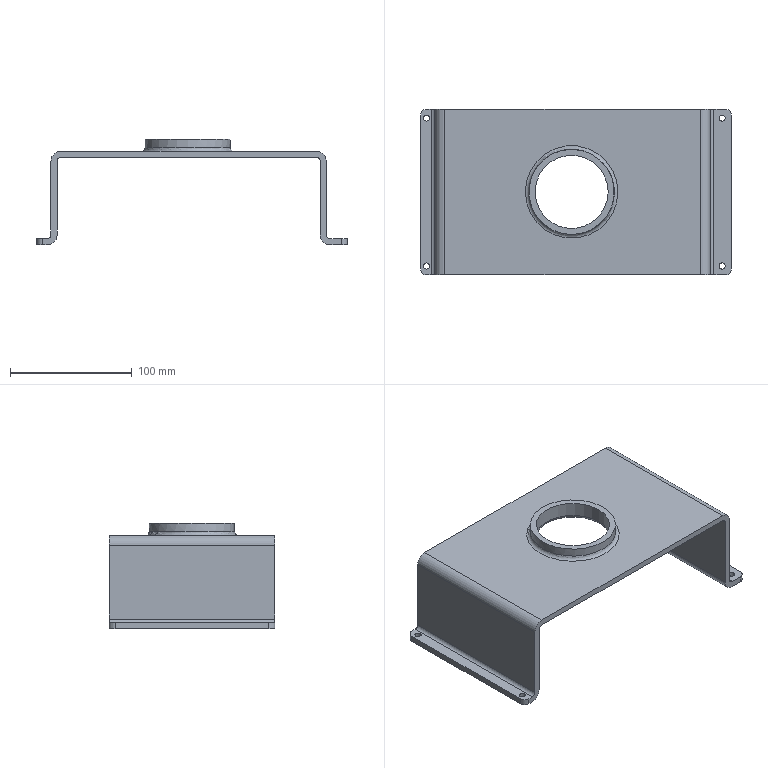Part | NX | features BREP 1 | 1 solid | 35 faces | box 255.4 x 136 x 86.7 mm | volume 260329 mm3 | cylinder 18 | plane 15 | torus 2 | commonest cylinder face diameters 5 x4 6 x4 10 x4 16 x4 60 x1 70 x1
STEP:
#1=CARTESIAN_POINT('',(38.,0.,5.));
#2=VERTEX_POINT('',#1);
#3=CARTESIAN_POINT('',(0.,0.,5.));
#4=DIRECTION('',(0.,0.,-1.));
#5=DIRECTION('',(1.,0.,0.));
#6=AXIS2_PLACEMENT_3D('',#3,#4,#5);
#7=CIRCLE('',#6,38.);
#8=EDGE_CURVE('',#2,#2,#7,.T.);
#9=ORIENTED_EDGE('',*,*,#8,.T.);
#10=EDGE_LOOP('',(#9));
#11=FACE_BOUND('',#10,.T.);
#12=CARTESIAN_POINT('',(-104.221,-68.,5.));
#13=VERTEX_POINT('',#12);
#14=CARTESIAN_POINT('',(105.779,-68.,5.));
#15=VERTEX_POINT('',#14);
#16=CARTESIAN_POINT('',(-124.221,-68.,5.));
#17=DIRECTION('',(1.,0.,0.));
#18=VECTOR('',#17,1000.);
#19=LINE('',#16,#18);
#20=EDGE_CURVE('',#13,#15,#19,.T.);
#21=ORIENTED_EDGE('',*,*,#20,.T.);
#22=CARTESIAN_POINT('',(105.779,68.,5.));
#23=VERTEX_POINT('',#22);
#24=CARTESIAN_POINT('',(105.779,-68.,5.));
#25=DIRECTION('',(0.,1.,0.));
#26=VECTOR('',#25,1000.);
#27=LINE('',#24,#26);
#28=EDGE_CURVE('',#15,#23,#27,.T.);
#29=ORIENTED_EDGE('',*,*,#28,.T.);
#30=CARTESIAN_POINT('',(-104.221,68.,5.));
#31=VERTEX_POINT('',#30);
#32=CARTESIAN_POINT('',(131.779,68.,5.));
#33=DIRECTION('',(-1.,0.,0.));
#34=VECTOR('',#33,1000.);
#35=LINE('',#32,#34);
#36=EDGE_CURVE('',#23,#31,#35,.T.);
#37=ORIENTED_EDGE('',*,*,#36,.T.);
#38=CARTESIAN_POINT('',(-104.221,68.,5.));
#39=DIRECTION('',(0.,-1.,0.));
#40=VECTOR('',#39,1000.);
#41=LINE('',#38,#40);
#42=EDGE_CURVE('',#31,#13,#41,.T.);
#43=ORIENTED_EDGE('',*,*,#42,.T.);
#44=EDGE_LOOP('',(#21,#29,#37,#43));
#45=FACE_BOUND('',#44,.T.);
#46=CARTESIAN_POINT('',(0.,0.,5.));
#47=DIRECTION('',(0.,0.,1.));
#48=DIRECTION('',(-1.,0.,0.));
#49=AXIS2_PLACEMENT_3D('',#46,#47,#48);
#50=PLANE('',#49);
#51=ADVANCED_FACE('',(#11,#45),#50,.T.);
#52=CARTESIAN_POINT('',(-115.221,68.,-71.7));
#53=VERTEX_POINT('',#52);
#54=CARTESIAN_POINT('',(-119.121,68.,-71.7));
#55=VERTEX_POINT('',#54);
#56=CARTESIAN_POINT('',(-115.221,68.,-71.7));
#57=DIRECTION('',(-1.,0.,0.));
#58=VECTOR('',#57,1000.);
#59=LINE('',#56,#58);
#60=EDGE_CURVE('',#53,#55,#59,.T.);
#61=ORIENTED_EDGE('',*,*,#60,.T.);
#62=CARTESIAN_POINT('',(-119.121,68.,-66.7));
#63=VERTEX_POINT('',#62);
#64=CARTESIAN_POINT('',(-119.121,68.,-66.7));
#65=DIRECTION('',(0.,0.,1.));
#66=VECTOR('',#65,1000.);
#67=LINE('',#64,#66);
#68=EDGE_CURVE('',#55,#63,#67,.T.);
#69=ORIENTED_EDGE('',*,*,#68,.T.);
#70=CARTESIAN_POINT('',(-115.221,68.,-66.7));
#71=VERTEX_POINT('',#70);
#72=CARTESIAN_POINT('',(-115.221,68.,-66.7));
#73=DIRECTION('',(-1.,0.,0.));
#74=VECTOR('',#73,1000.);
#75=LINE('',#72,#74);
#76=EDGE_CURVE('',#71,#63,#75,.T.);
#77=ORIENTED_EDGE('',*,*,#76,.F.);
#78=CARTESIAN_POINT('',(-112.221,68.,-63.7));
#79=VERTEX_POINT('',#78);
#80=CARTESIAN_POINT('',(-115.221,68.,-63.7));
#81=DIRECTION('',(0.,1.,0.));
#82=DIRECTION('',(1.,0.,0.));
#83=AXIS2_PLACEMENT_3D('',#80,#81,#82);
#84=CIRCLE('',#83,3.);
#85=EDGE_CURVE('',#79,#71,#84,.T.);
#86=ORIENTED_EDGE('',*,*,#85,.F.);
#87=CARTESIAN_POINT('',(-112.221,68.,-3.));
#88=VERTEX_POINT('',#87);
#89=CARTESIAN_POINT('',(-112.221,68.,-3.));
#90=DIRECTION('',(0.,0.,-1.));
#91=VECTOR('',#90,1000.);
#92=LINE('',#89,#91);
#93=EDGE_CURVE('',#88,#79,#92,.T.);
#94=ORIENTED_EDGE('',*,*,#93,.F.);
#95=CARTESIAN_POINT('',(-104.221,68.,-3.));
#96=DIRECTION('',(0.,-1.,0.));
#97=DIRECTION('',(-1.,0.,0.));
#98=AXIS2_PLACEMENT_3D('',#95,#96,#97);
#99=CIRCLE('',#98,8.);
#100=EDGE_CURVE('',#31,#88,#99,.T.);
#101=ORIENTED_EDGE('',*,*,#100,.F.);
#102=ORIENTED_EDGE('',*,*,#36,.F.);
#103=CARTESIAN_POINT('',(113.779,68.,-3.));
#104=VERTEX_POINT('',#103);
#105=CARTESIAN_POINT('',(105.779,68.,-3.));
#106=DIRECTION('',(0.,1.,0.));
#107=DIRECTION('',(1.,0.,0.));
#108=AXIS2_PLACEMENT_3D('',#105,#106,#107);
#109=CIRCLE('',#108,8.);
#110=EDGE_CURVE('',#23,#104,#109,.T.);
#111=ORIENTED_EDGE('',*,*,#110,.T.);
#112=CARTESIAN_POINT('',(113.779,68.,-63.6));
#113=VERTEX_POINT('',#112);
#114=CARTESIAN_POINT('',(113.779,68.,-3.));
#115=DIRECTION('',(0.,0.,-1.));
#116=VECTOR('',#115,1000.);
#117=LINE('',#114,#116);
#118=EDGE_CURVE('',#104,#113,#117,.T.);
#119=ORIENTED_EDGE('',*,*,#118,.T.);
#120=CARTESIAN_POINT('',(116.779,68.,-66.6));
#121=VERTEX_POINT('',#120);
#122=CARTESIAN_POINT('',(116.779,68.,-63.6));
#123=DIRECTION('',(0.,-1.,0.));
#124=DIRECTION('',(-1.,0.,0.));
#125=AXIS2_PLACEMENT_3D('',#122,#123,#124);
#126=CIRCLE('',#125,3.);
#127=EDGE_CURVE('',#113,#121,#126,.T.);
#128=ORIENTED_EDGE('',*,*,#127,.T.);
#129=CARTESIAN_POINT('',(126.279,68.,-66.6));
#130=VERTEX_POINT('',#129);
#131=CARTESIAN_POINT('',(116.779,68.,-66.6));
#132=DIRECTION('',(1.,0.,0.));
#133=VECTOR('',#132,1000.);
#134=LINE('',#131,#133);
#135=EDGE_CURVE('',#121,#130,#134,.T.);
#136=ORIENTED_EDGE('',*,*,#135,.T.);
#137=CARTESIAN_POINT('',(126.279,68.,-71.6));
#138=VERTEX_POINT('',#137);
#139=CARTESIAN_POINT('',(126.279,68.,-71.6));
#140=DIRECTION('',(0.,0.,-1.));
#141=VECTOR('',#140,1000.);
#142=LINE('',#139,#141);
#143=EDGE_CURVE('',#130,#138,#142,.T.);
#144=ORIENTED_EDGE('',*,*,#143,.T.);
#145=CARTESIAN_POINT('',(116.779,68.,-71.6));
#146=VERTEX_POINT('',#145);
#147=CARTESIAN_POINT('',(116.779,68.,-71.6));
#148=DIRECTION('',(1.,0.,0.));
#149=VECTOR('',#148,1000.);
#150=LINE('',#147,#149);
#151=EDGE_CURVE('',#146,#138,#150,.T.);
#152=ORIENTED_EDGE('',*,*,#151,.F.);
#153=CARTESIAN_POINT('',(108.779,68.,-63.6));
#154=VERTEX_POINT('',#153);
#155=CARTESIAN_POINT('',(116.779,68.,-63.6));
#156=DIRECTION('',(0.,-1.,0.));
#157=DIRECTION('',(-1.,0.,0.));
#158=AXIS2_PLACEMENT_3D('',#155,#156,#157);
#159=CIRCLE('',#158,8.);
#160=EDGE_CURVE('',#154,#146,#159,.T.);
#161=ORIENTED_EDGE('',*,*,#160,.F.);
#162=CARTESIAN_POINT('',(108.779,68.,-3.));
#163=VERTEX_POINT('',#162);
#164=CARTESIAN_POINT('',(108.779,68.,-3.));
#165=DIRECTION('',(0.,0.,-1.));
#166=VECTOR('',#165,1000.);
#167=LINE('',#164,#166);
#168=EDGE_CURVE('',#163,#154,#167,.T.);
#169=ORIENTED_EDGE('',*,*,#168,.F.);
#170=CARTESIAN_POINT('',(105.779,68.,0.));
#171=VERTEX_POINT('',#170);
#172=CARTESIAN_POINT('',(105.779,68.,-3.));
#173=DIRECTION('',(0.,1.,0.));
#174=DIRECTION('',(0.,0.,1.));
#175=AXIS2_PLACEMENT_3D('',#172,#173,#174);
#176=CIRCLE('',#175,3.);
#177=EDGE_CURVE('',#171,#163,#176,.T.);
#178=ORIENTED_EDGE('',*,*,#177,.F.);
#179=CARTESIAN_POINT('',(-104.221,68.,0.));
#180=VERTEX_POINT('',#179);
#181=CARTESIAN_POINT('',(0.,68.,0.));
#182=DIRECTION('',(-1.,0.,0.));
#183=VECTOR('',#182,1000.);
#184=LINE('',#181,#183);
#185=EDGE_CURVE('',#171,#180,#184,.T.);
#186=ORIENTED_EDGE('',*,*,#185,.T.);
#187=CARTESIAN_POINT('',(-107.221,68.,-3.));
#188=VERTEX_POINT('',#187);
#189=CARTESIAN_POINT('',(-104.221,68.,-3.));
#190=DIRECTION('',(0.,-1.,0.));
#191=DIRECTION('',(0.,0.,1.));
#192=AXIS2_PLACEMENT_3D('',#189,#190,#191);
#193=CIRCLE('',#192,3.);
#194=EDGE_CURVE('',#180,#188,#193,.T.);
#195=ORIENTED_EDGE('',*,*,#194,.T.);
#196=CARTESIAN_POINT('',(-107.221,68.,-63.7));
#197=VERTEX_POINT('',#196);
#198=CARTESIAN_POINT('',(-107.221,68.,-3.));
#199=DIRECTION('',(0.,0.,-1.));
#200=VECTOR('',#199,1000.);
#201=LINE('',#198,#200);
#202=EDGE_CURVE('',#188,#197,#201,.T.);
#203=ORIENTED_EDGE('',*,*,#202,.T.);
#204=CARTESIAN_POINT('',(-115.221,68.,-63.7));
#205=DIRECTION('',(0.,1.,0.));
#206=DIRECTION('',(1.,0.,0.));
#207=AXIS2_PLACEMENT_3D('',#204,#205,#206);
#208=CIRCLE('',#207,8.);
#209=EDGE_CURVE('',#197,#53,#208,.T.);
#210=ORIENTED_EDGE('',*,*,#209,.T.);
#211=EDGE_LOOP('',(#61,#69,#77,#86,#94,#101,#102,#111,#119,#128,#136,#144,#152,#161,#169,#178,#186,#195,#203,#210));
#212=FACE_BOUND('',#211,.T.);
#213=CARTESIAN_POINT('',(0.,68.,5.));
#214=DIRECTION('',(0.,-1.,0.));
#215=DIRECTION('',(-1.,0.,0.));
#216=AXIS2_PLACEMENT_3D('',#213,#214,#215);
#217=PLANE('',#216);
#218=ADVANCED_FACE('',(#212),#217,.F.);
#219=CARTESIAN_POINT('',(-115.221,-68.,-66.7));
#220=VERTEX_POINT('',#219);
#221=CARTESIAN_POINT('',(-119.121,-68.,-66.7));
#222=VERTEX_POINT('',#221);
#223=CARTESIAN_POINT('',(-115.221,-68.,-66.7));
#224=DIRECTION('',(-1.,0.,0.));
#225=VECTOR('',#224,1000.);
#226=LINE('',#223,#225);
#227=EDGE_CURVE('',#220,#222,#226,.T.);
#228=ORIENTED_EDGE('',*,*,#227,.T.);
#229=CARTESIAN_POINT('',(-119.121,-68.,-71.7));
#230=VERTEX_POINT('',#229);
#231=CARTESIAN_POINT('',(-119.121,-68.,-71.7));
#232=DIRECTION('',(0.,0.,-1.));
#233=VECTOR('',#232,1000.);
#234=LINE('',#231,#233);
#235=EDGE_CURVE('',#222,#230,#234,.T.);
#236=ORIENTED_EDGE('',*,*,#235,.T.);
#237=CARTESIAN_POINT('',(-115.221,-68.,-71.7));
#238=VERTEX_POINT('',#237);
#239=CARTESIAN_POINT('',(-115.221,-68.,-71.7));
#240=DIRECTION('',(-1.,0.,0.));
#241=VECTOR('',#240,1000.);
#242=LINE('',#239,#241);
#243=EDGE_CURVE('',#238,#230,#242,.T.);
#244=ORIENTED_EDGE('',*,*,#243,.F.);
#245=CARTESIAN_POINT('',(-107.221,-68.,-63.7));
#246=VERTEX_POINT('',#245);
#247=CARTESIAN_POINT('',(-115.221,-68.,-63.7));
#248=DIRECTION('',(0.,1.,0.));
#249=DIRECTION('',(1.,0.,0.));
#250=AXIS2_PLACEMENT_3D('',#247,#248,#249);
#251=CIRCLE('',#250,8.);
#252=EDGE_CURVE('',#246,#238,#251,.T.);
#253=ORIENTED_EDGE('',*,*,#252,.F.);
#254=CARTESIAN_POINT('',(-107.221,-68.,-3.));
#255=VERTEX_POINT('',#254);
#256=CARTESIAN_POINT('',(-107.221,-68.,-3.));
#257=DIRECTION('',(0.,0.,-1.));
#258=VECTOR('',#257,1000.);
#259=LINE('',#256,#258);
#260=EDGE_CURVE('',#255,#246,#259,.T.);
#261=ORIENTED_EDGE('',*,*,#260,.F.);
#262=CARTESIAN_POINT('',(-104.221,-68.,0.));
#263=VERTEX_POINT('',#262);
#264=CARTESIAN_POINT('',(-104.221,-68.,-3.));
#265=DIRECTION('',(0.,-1.,0.));
#266=DIRECTION('',(0.,0.,1.));
#267=AXIS2_PLACEMENT_3D('',#264,#265,#266);
#268=CIRCLE('',#267,3.);
#269=EDGE_CURVE('',#263,#255,#268,.T.);
#270=ORIENTED_EDGE('',*,*,#269,.F.);
#271=CARTESIAN_POINT('',(105.779,-68.,0.));
#272=VERTEX_POINT('',#271);
#273=CARTESIAN_POINT('',(-124.221,-68.,0.));
#274=DIRECTION('',(1.,0.,0.));
#275=VECTOR('',#274,1000.);
#276=LINE('',#273,#275);
#277=EDGE_CURVE('',#263,#272,#276,.T.);
#278=ORIENTED_EDGE('',*,*,#277,.T.);
#279=CARTESIAN_POINT('',(108.779,-68.,-3.));
#280=VERTEX_POINT('',#279);
#281=CARTESIAN_POINT('',(105.779,-68.,-3.));
#282=DIRECTION('',(0.,1.,0.));
#283=DIRECTION('',(0.,0.,1.));
#284=AXIS2_PLACEMENT_3D('',#281,#282,#283);
#285=CIRCLE('',#284,3.);
#286=EDGE_CURVE('',#272,#280,#285,.T.);
#287=ORIENTED_EDGE('',*,*,#286,.T.);
#288=CARTESIAN_POINT('',(108.779,-68.,-63.6));
#289=VERTEX_POINT('',#288);
#290=CARTESIAN_POINT('',(108.779,-68.,-3.));
#291=DIRECTION('',(0.,0.,-1.));
#292=VECTOR('',#291,1000.);
#293=LINE('',#290,#292);
#294=EDGE_CURVE('',#280,#289,#293,.T.);
#295=ORIENTED_EDGE('',*,*,#294,.T.);
#296=CARTESIAN_POINT('',(116.779,-68.,-71.6));
#297=VERTEX_POINT('',#296);
#298=CARTESIAN_POINT('',(116.779,-68.,-63.6));
#299=DIRECTION('',(0.,-1.,0.));
#300=DIRECTION('',(-1.,0.,0.));
#301=AXIS2_PLACEMENT_3D('',#298,#299,#300);
#302=CIRCLE('',#301,8.);
#303=EDGE_CURVE('',#289,#297,#302,.T.);
#304=ORIENTED_EDGE('',*,*,#303,.T.);
#305=CARTESIAN_POINT('',(126.279,-68.,-71.6));
#306=VERTEX_POINT('',#305);
#307=CARTESIAN_POINT('',(116.779,-68.,-71.6));
#308=DIRECTION('',(1.,0.,0.));
#309=VECTOR('',#308,1000.);
#310=LINE('',#307,#309);
#311=EDGE_CURVE('',#297,#306,#310,.T.);
#312=ORIENTED_EDGE('',*,*,#311,.T.);
#313=CARTESIAN_POINT('',(126.279,-68.,-66.6));
#314=VERTEX_POINT('',#313);
#315=CARTESIAN_POINT('',(126.279,-68.,-66.6));
#316=DIRECTION('',(0.,0.,1.));
#317=VECTOR('',#316,1000.);
#318=LINE('',#315,#317);
#319=EDGE_CURVE('',#306,#314,#318,.T.);
#320=ORIENTED_EDGE('',*,*,#319,.T.);
#321=CARTESIAN_POINT('',(116.779,-68.,-66.6));
#322=VERTEX_POINT('',#321);
#323=CARTESIAN_POINT('',(116.779,-68.,-66.6));
#324=DIRECTION('',(1.,0.,0.));
#325=VECTOR('',#324,1000.);
#326=LINE('',#323,#325);
#327=EDGE_CURVE('',#322,#314,#326,.T.);
#328=ORIENTED_EDGE('',*,*,#327,.F.);
#329=CARTESIAN_POINT('',(113.779,-68.,-63.6));
#330=VERTEX_POINT('',#329);
#331=CARTESIAN_POINT('',(116.779,-68.,-63.6));
#332=DIRECTION('',(0.,-1.,0.));
#333=DIRECTION('',(-1.,0.,0.));
#334=AXIS2_PLACEMENT_3D('',#331,#332,#333);
#335=CIRCLE('',#334,3.);
#336=EDGE_CURVE('',#330,#322,#335,.T.);
#337=ORIENTED_EDGE('',*,*,#336,.F.);
#338=CARTESIAN_POINT('',(113.779,-68.,-3.));
#339=VERTEX_POINT('',#338);
#340=CARTESIAN_POINT('',(113.779,-68.,-3.));
#341=DIRECTION('',(0.,0.,-1.));
#342=VECTOR('',#341,1000.);
#343=LINE('',#340,#342);
#344=EDGE_CURVE('',#339,#330,#343,.T.);
#345=ORIENTED_EDGE('',*,*,#344,.F.);
#346=CARTESIAN_POINT('',(105.779,-68.,-3.));
#347=DIRECTION('',(0.,1.,0.));
#348=DIRECTION('',(1.,0.,0.));
#349=AXIS2_PLACEMENT_3D('',#346,#347,#348);
#350=CIRCLE('',#349,8.);
#351=EDGE_CURVE('',#15,#339,#350,.T.);
#352=ORIENTED_EDGE('',*,*,#351,.F.);
#353=ORIENTED_EDGE('',*,*,#20,.F.);
#354=CARTESIAN_POINT('',(-112.221,-68.,-3.));
#355=VERTEX_POINT('',#354);
#356=CARTESIAN_POINT('',(-104.221,-68.,-3.));
#357=DIRECTION('',(0.,-1.,0.));
#358=DIRECTION('',(-1.,0.,0.));
#359=AXIS2_PLACEMENT_3D('',#356,#357,#358);
#360=CIRCLE('',#359,8.);
#361=EDGE_CURVE('',#13,#355,#360,.T.);
#362=ORIENTED_EDGE('',*,*,#361,.T.);
#363=CARTESIAN_POINT('',(-112.221,-68.,-63.7));
#364=VERTEX_POINT('',#363);
#365=CARTESIAN_POINT('',(-112.221,-68.,-3.));
#366=DIRECTION('',(0.,0.,-1.));
#367=VECTOR('',#366,1000.);
#368=LINE('',#365,#367);
#369=EDGE_CURVE('',#355,#364,#368,.T.);
#370=ORIENTED_EDGE('',*,*,#369,.T.);
#371=CARTESIAN_POINT('',(-115.221,-68.,-63.7));
#372=DIRECTION('',(0.,1.,0.));
#373=DIRECTION('',(1.,0.,0.));
#374=AXIS2_PLACEMENT_3D('',#371,#372,#373);
#375=CIRCLE('',#374,3.);
#376=EDGE_CURVE('',#364,#220,#375,.T.);
#377=ORIENTED_EDGE('',*,*,#376,.T.);
#378=EDGE_LOOP('',(#228,#236,#244,#253,#261,#270,#278,#287,#295,#304,#312,#320,#328,#337,#345,#352,#353,#362,#370,#377));
#379=FACE_BOUND('',#378,.T.);
#380=CARTESIAN_POINT('',(-124.221,-68.,5.));
#381=DIRECTION('',(0.,1.,0.));
#382=DIRECTION('',(1.,0.,0.));
#383=AXIS2_PLACEMENT_3D('',#380,#381,#382);
#384=PLANE('',#383);
#385=ADVANCED_FACE('',(#379),#384,.F.);
#386=CARTESIAN_POINT('',(33.,0.,0.));
#387=VERTEX_POINT('',#386);
#388=CARTESIAN_POINT('',(0.,0.,0.));
#389=DIRECTION('',(0.,0.,1.));
#390=DIRECTION('',(1.,0.,0.));
#391=AXIS2_PLACEMENT_3D('',#388,#389,#390);
#392=CIRCLE('',#391,33.);
#393=EDGE_CURVE('',#387,#387,#392,.T.);
#394=ORIENTED_EDGE('',*,*,#393,.T.);
#395=EDGE_LOOP('',(#394));
#396=FACE_BOUND('',#395,.T.);
#397=CARTESIAN_POINT('',(105.779,-68.,0.));
#398=DIRECTION('',(0.,1.,0.));
#399=VECTOR('',#398,1000.);
#400=LINE('',#397,#399);
#401=EDGE_CURVE('',#272,#171,#400,.T.);
#402=ORIENTED_EDGE('',*,*,#401,.F.);
#403=ORIENTED_EDGE('',*,*,#277,.F.);
#404=CARTESIAN_POINT('',(-104.221,68.,0.));
#405=DIRECTION('',(0.,-1.,0.));
#406=VECTOR('',#405,1000.);
#407=LINE('',#404,#406);
#408=EDGE_CURVE('',#180,#263,#407,.T.);
#409=ORIENTED_EDGE('',*,*,#408,.F.);
#410=ORIENTED_EDGE('',*,*,#185,.F.);
#411=EDGE_LOOP('',(#402,#403,#409,#410));
#412=FACE_BOUND('',#411,.T.);
#413=CARTESIAN_POINT('',(0.,0.,0.));
#414=DIRECTION('',(0.,0.,1.));
#415=DIRECTION('',(-1.,0.,0.));
#416=AXIS2_PLACEMENT_3D('',#413,#414,#415);
#417=PLANE('',#416);
#418=ADVANCED_FACE('',(#396,#412),#417,.F.);
#419=ORIENTED_EDGE('',*,*,#286,.F.);
#420=ORIENTED_EDGE('',*,*,#401,.T.);
#421=ORIENTED_EDGE('',*,*,#177,.T.);
#422=CARTESIAN_POINT('',(108.779,68.,-3.));
#423=DIRECTION('',(0.,-1.,0.));
#424=VECTOR('',#423,1000.);
#425=LINE('',#422,#424);
#426=EDGE_CURVE('',#163,#280,#425,.T.);
#427=ORIENTED_EDGE('',*,*,#426,.T.);
#428=EDGE_LOOP('',(#419,#420,#421,#427));
#429=FACE_BOUND('',#428,.T.);
#430=CARTESIAN_POINT('',(105.779,68.,-3.));
#431=DIRECTION('',(0.,-1.,0.));
#432=DIRECTION('',(-1.,0.,0.));
#433=AXIS2_PLACEMENT_3D('',#430,#431,#432);
#434=CYLINDRICAL_SURFACE('',#433,3.);
#435=ADVANCED_FACE('',(#429),#434,.F.);
#436=ORIENTED_EDGE('',*,*,#294,.F.);
#437=ORIENTED_EDGE('',*,*,#426,.F.);
#438=ORIENTED_EDGE('',*,*,#168,.T.);
#439=CARTESIAN_POINT('',(108.779,68.,-63.6));
#440=DIRECTION('',(0.,-1.,0.));
#441=VECTOR('',#440,1000.);
#442=LINE('',#439,#441);
#443=EDGE_CURVE('',#154,#289,#442,.T.);
#444=ORIENTED_EDGE('',*,*,#443,.T.);
#445=EDGE_LOOP('',(#436,#437,#438,#444));
#446=FACE_BOUND('',#445,.T.);
#447=CARTESIAN_POINT('',(108.779,68.,-3.));
#448=DIRECTION('',(-1.,0.,0.));
#449=DIRECTION('',(0.,1.,0.));
#450=AXIS2_PLACEMENT_3D('',#447,#448,#449);
#451=PLANE('',#450);
#452=ADVANCED_FACE('',(#446),#451,.T.);
#453=ORIENTED_EDGE('',*,*,#351,.T.);
#454=CARTESIAN_POINT('',(113.779,68.,-3.));
#455=DIRECTION('',(0.,-1.,0.));
#456=VECTOR('',#455,1000.);
#457=LINE('',#454,#456);
#458=EDGE_CURVE('',#104,#339,#457,.T.);
#459=ORIENTED_EDGE('',*,*,#458,.F.);
#460=ORIENTED_EDGE('',*,*,#110,.F.);
#461=ORIENTED_EDGE('',*,*,#28,.F.);
#462=EDGE_LOOP('',(#453,#459,#460,#461));
#463=FACE_BOUND('',#462,.T.);
#464=CARTESIAN_POINT('',(105.779,68.,-3.));
#465=DIRECTION('',(0.,-1.,0.));
#466=DIRECTION('',(-1.,0.,0.));
#467=AXIS2_PLACEMENT_3D('',#464,#465,#466);
#468=CYLINDRICAL_SURFACE('',#467,8.);
#469=ADVANCED_FACE('',(#463),#468,.T.);
#470=ORIENTED_EDGE('',*,*,#344,.T.);
#471=CARTESIAN_POINT('',(113.779,68.,-63.6));
#472=DIRECTION('',(0.,-1.,0.));
#473=VECTOR('',#472,1000.);
#474=LINE('',#471,#473);
#475=EDGE_CURVE('',#113,#330,#474,.T.);
#476=ORIENTED_EDGE('',*,*,#475,.F.);
#477=ORIENTED_EDGE('',*,*,#118,.F.);
#478=ORIENTED_EDGE('',*,*,#458,.T.);
#479=EDGE_LOOP('',(#470,#476,#477,#478));
#480=FACE_BOUND('',#479,.T.);
#481=CARTESIAN_POINT('',(113.779,68.,-3.));
#482=DIRECTION('',(-1.,0.,0.));
#483=DIRECTION('',(0.,1.,0.));
#484=AXIS2_PLACEMENT_3D('',#481,#482,#483);
#485=PLANE('',#484);
#486=ADVANCED_FACE('',(#480),#485,.F.);
#487=ORIENTED_EDGE('',*,*,#194,.F.);
#488=ORIENTED_EDGE('',*,*,#408,.T.);
#489=ORIENTED_EDGE('',*,*,#269,.T.);
#490=CARTESIAN_POINT('',(-107.221,-68.,-3.));
#491=DIRECTION('',(0.,1.,0.));
#492=VECTOR('',#491,1000.);
#493=LINE('',#490,#492);
#494=EDGE_CURVE('',#255,#188,#493,.T.);
#495=ORIENTED_EDGE('',*,*,#494,.T.);
#496=EDGE_LOOP('',(#487,#488,#489,#495));
#497=FACE_BOUND('',#496,.T.);
#498=CARTESIAN_POINT('',(-104.221,-68.,-3.));
#499=DIRECTION('',(0.,1.,0.));
#500=DIRECTION('',(1.,0.,0.));
#501=AXIS2_PLACEMENT_3D('',#498,#499,#500);
#502=CYLINDRICAL_SURFACE('',#501,3.);
#503=ADVANCED_FACE('',(#497),#502,.F.);
#504=ORIENTED_EDGE('',*,*,#202,.F.);
#505=ORIENTED_EDGE('',*,*,#494,.F.);
#506=ORIENTED_EDGE('',*,*,#260,.T.);
#507=CARTESIAN_POINT('',(-107.221,-68.,-63.7));
#508=DIRECTION('',(0.,1.,0.));
#509=VECTOR('',#508,1000.);
#510=LINE('',#507,#509);
#511=EDGE_CURVE('',#246,#197,#510,.T.);
#512=ORIENTED_EDGE('',*,*,#511,.T.);
#513=EDGE_LOOP('',(#504,#505,#506,#512));
#514=FACE_BOUND('',#513,.T.);
#515=CARTESIAN_POINT('',(-107.221,-68.,-3.));
#516=DIRECTION('',(1.,0.,0.));
#517=DIRECTION('',(0.,-1.,0.));
#518=AXIS2_PLACEMENT_3D('',#515,#516,#517);
#519=PLANE('',#518);
#520=ADVANCED_FACE('',(#514),#519,.T.);
#521=ORIENTED_EDGE('',*,*,#100,.T.);
#522=CARTESIAN_POINT('',(-112.221,-68.,-3.));
#523=DIRECTION('',(0.,1.,0.));
#524=VECTOR('',#523,1000.);
#525=LINE('',#522,#524);
#526=EDGE_CURVE('',#355,#88,#525,.T.);
#527=ORIENTED_EDGE('',*,*,#526,.F.);
#528=ORIENTED_EDGE('',*,*,#361,.F.);
#529=ORIENTED_EDGE('',*,*,#42,.F.);
#530=EDGE_LOOP('',(#521,#527,#528,#529));
#531=FACE_BOUND('',#530,.T.);
#532=CARTESIAN_POINT('',(-104.221,-68.,-3.));
#533=DIRECTION('',(0.,1.,0.));
#534=DIRECTION('',(1.,0.,0.));
#535=AXIS2_PLACEMENT_3D('',#532,#533,#534);
#536=CYLINDRICAL_SURFACE('',#535,8.);
#537=ADVANCED_FACE('',(#531),#536,.T.);
#538=ORIENTED_EDGE('',*,*,#93,.T.);
#539=CARTESIAN_POINT('',(-112.221,-68.,-63.7));
#540=DIRECTION('',(0.,1.,0.));
#541=VECTOR('',#540,1000.);
#542=LINE('',#539,#541);
#543=EDGE_CURVE('',#364,#79,#542,.T.);
#544=ORIENTED_EDGE('',*,*,#543,.F.);
#545=ORIENTED_EDGE('',*,*,#369,.F.);
#546=ORIENTED_EDGE('',*,*,#526,.T.);
#547=EDGE_LOOP('',(#538,#544,#545,#546));
#548=FACE_BOUND('',#547,.T.);
#549=CARTESIAN_POINT('',(-112.221,-68.,-3.));
#550=DIRECTION('',(1.,0.,0.));
#551=DIRECTION('',(0.,-1.,0.));
#552=AXIS2_PLACEMENT_3D('',#549,#550,#551);
#553=PLANE('',#552);
#554=ADVANCED_FACE('',(#548),#553,.F.);
#555=CARTESIAN_POINT('',(131.279,-63.,-66.6));
#556=VERTEX_POINT('',#555);
#557=CARTESIAN_POINT('',(131.279,63.,-66.6));
#558=VERTEX_POINT('',#557);
#559=CARTESIAN_POINT('',(131.279,-68.,-66.6));
#560=DIRECTION('',(0.,1.,0.));
#561=VECTOR('',#560,1000.);
#562=LINE('',#559,#561);
#563=EDGE_CURVE('',#556,#558,#562,.T.);
#564=ORIENTED_EDGE('',*,*,#563,.F.);
#565=CARTESIAN_POINT('',(131.279,-63.,-71.6));
#566=VERTEX_POINT('',#565);
#567=CARTESIAN_POINT('',(131.279,-63.,-71.6));
#568=DIRECTION('',(0.,0.,-1.));
#569=VECTOR('',#568,1000.);
#570=LINE('',#567,#569);
#571=EDGE_CURVE('',#556,#566,#570,.T.);
#572=ORIENTED_EDGE('',*,*,#571,.T.);
#573=CARTESIAN_POINT('',(131.279,63.,-71.6));
#574=VERTEX_POINT('',#573);
#575=CARTESIAN_POINT('',(131.279,-68.,-71.6));
#576=DIRECTION('',(0.,1.,0.));
#577=VECTOR('',#576,1000.);
#578=LINE('',#575,#577);
#579=EDGE_CURVE('',#566,#574,#578,.T.);
#580=ORIENTED_EDGE('',*,*,#579,.T.);
#581=CARTESIAN_POINT('',(131.279,63.,-66.6));
#582=DIRECTION('',(0.,0.,1.));
#583=VECTOR('',#582,1000.);
#584=LINE('',#581,#583);
#585=EDGE_CURVE('',#574,#558,#584,.T.);
#586=ORIENTED_EDGE('',*,*,#585,.T.);
#587=EDGE_LOOP('',(#564,#572,#580,#586));
#588=FACE_BOUND('',#587,.T.);
#589=CARTESIAN_POINT('',(131.279,-68.,-66.6));
#590=DIRECTION('',(1.,0.,0.));
#591=DIRECTION('',(0.,-1.,0.));
#592=AXIS2_PLACEMENT_3D('',#589,#590,#591);
#593=PLANE('',#592);
#594=ADVANCED_FACE('',(#588),#593,.T.);
#595=ORIENTED_EDGE('',*,*,#127,.F.);
#596=ORIENTED_EDGE('',*,*,#475,.T.);
#597=ORIENTED_EDGE('',*,*,#336,.T.);
#598=CARTESIAN_POINT('',(116.779,-68.,-66.6));
#599=DIRECTION('',(0.,1.,0.));
#600=VECTOR('',#599,1000.);
#601=LINE('',#598,#600);
#602=EDGE_CURVE('',#322,#121,#601,.T.);
#603=ORIENTED_EDGE('',*,*,#602,.T.);
#604=EDGE_LOOP('',(#595,#596,#597,#603));
#605=FACE_BOUND('',#604,.T.);
#606=CARTESIAN_POINT('',(116.779,-68.,-63.6));
#607=DIRECTION('',(0.,1.,0.));
#608=DIRECTION('',(1.,0.,0.));
#609=AXIS2_PLACEMENT_3D('',#606,#607,#608);
#610=CYLINDRICAL_SURFACE('',#609,3.);
#611=ADVANCED_FACE('',(#605),#610,.F.);
#612=CARTESIAN_POINT('',(126.047,-60.702,-66.6));
#613=VERTEX_POINT('',#612);
#614=CARTESIAN_POINT('',(123.547,-60.702,-66.6));
#615=DIRECTION('',(0.,0.,1.));
#616=DIRECTION('',(1.,0.,0.));
#617=AXIS2_PLACEMENT_3D('',#614,#615,#616);
#618=CIRCLE('',#617,2.5);
#619=EDGE_CURVE('',#613,#613,#618,.T.);
#620=ORIENTED_EDGE('',*,*,#619,.F.);
#621=EDGE_LOOP('',(#620));
#622=FACE_BOUND('',#621,.T.);
#623=CARTESIAN_POINT('',(126.047,60.702,-66.6));
#624=VERTEX_POINT('',#623);
#625=CARTESIAN_POINT('',(123.547,60.702,-66.6));
#626=DIRECTION('',(0.,0.,1.));
#627=DIRECTION('',(1.,0.,0.));
#628=AXIS2_PLACEMENT_3D('',#625,#626,#627);
#629=CIRCLE('',#628,2.5);
#630=EDGE_CURVE('',#624,#624,#629,.T.);
#631=ORIENTED_EDGE('',*,*,#630,.F.);
#632=EDGE_LOOP('',(#631));
#633=FACE_BOUND('',#632,.T.);
#634=ORIENTED_EDGE('',*,*,#327,.T.);
#635=CARTESIAN_POINT('',(126.279,-63.,-66.6));
#636=DIRECTION('',(0.,0.,1.));
#637=DIRECTION('',(1.,0.,0.));
#638=AXIS2_PLACEMENT_3D('',#635,#636,#637);
#639=CIRCLE('',#638,5.);
#640=EDGE_CURVE('',#314,#556,#639,.T.);
#641=ORIENTED_EDGE('',*,*,#640,.T.);
#642=ORIENTED_EDGE('',*,*,#563,.T.);
#643=CARTESIAN_POINT('',(126.279,63.,-66.6));
#644=DIRECTION('',(0.,0.,1.));
#645=DIRECTION('',(1.,0.,0.));
#646=AXIS2_PLACEMENT_3D('',#643,#644,#645);
#647=CIRCLE('',#646,5.);
#648=EDGE_CURVE('',#558,#130,#647,.T.);
#649=ORIENTED_EDGE('',*,*,#648,.T.);
#650=ORIENTED_EDGE('',*,*,#135,.F.);
#651=ORIENTED_EDGE('',*,*,#602,.F.);
#652=EDGE_LOOP('',(#634,#641,#642,#649,#650,#651));
#653=FACE_BOUND('',#652,.T.);
#654=CARTESIAN_POINT('',(116.779,-68.,-66.6));
#655=DIRECTION('',(0.,0.,1.));
#656=DIRECTION('',(-1.,0.,0.));
#657=AXIS2_PLACEMENT_3D('',#654,#655,#656);
#658=PLANE('',#657);
#659=ADVANCED_FACE('',(#622,#633,#653),#658,.T.);
#660=ORIENTED_EDGE('',*,*,#160,.T.);
#661=CARTESIAN_POINT('',(116.779,-68.,-71.6));
#662=DIRECTION('',(0.,1.,0.));
#663=VECTOR('',#662,1000.);
#664=LINE('',#661,#663);
#665=EDGE_CURVE('',#297,#146,#664,.T.);
#666=ORIENTED_EDGE('',*,*,#665,.F.);
#667=ORIENTED_EDGE('',*,*,#303,.F.);
#668=ORIENTED_EDGE('',*,*,#443,.F.);
#669=EDGE_LOOP('',(#660,#666,#667,#668));
#670=FACE_BOUND('',#669,.T.);
#671=CARTESIAN_POINT('',(116.779,-68.,-63.6));
#672=DIRECTION('',(0.,1.,0.));
#673=DIRECTION('',(1.,0.,0.));
#674=AXIS2_PLACEMENT_3D('',#671,#672,#673);
#675=CYLINDRICAL_SURFACE('',#674,8.);
#676=ADVANCED_FACE('',(#670),#675,.T.);
#677=CARTESIAN_POINT('',(126.047,-60.702,-71.6));
#678=VERTEX_POINT('',#677);
#679=CARTESIAN_POINT('',(123.547,-60.702,-71.6));
#680=DIRECTION('',(0.,0.,1.));
#681=DIRECTION('',(1.,0.,0.));
#682=AXIS2_PLACEMENT_3D('',#679,#680,#681);
#683=CIRCLE('',#682,2.5);
#684=EDGE_CURVE('',#678,#678,#683,.T.);
#685=ORIENTED_EDGE('',*,*,#684,.T.);
#686=EDGE_LOOP('',(#685));
#687=FACE_BOUND('',#686,.T.);
#688=CARTESIAN_POINT('',(126.047,60.702,-71.6));
#689=VERTEX_POINT('',#688);
#690=CARTESIAN_POINT('',(123.547,60.702,-71.6));
#691=DIRECTION('',(0.,0.,1.));
#692=DIRECTION('',(1.,0.,0.));
#693=AXIS2_PLACEMENT_3D('',#690,#691,#692);
#694=CIRCLE('',#693,2.5);
#695=EDGE_CURVE('',#689,#689,#694,.T.);
#696=ORIENTED_EDGE('',*,*,#695,.T.);
#697=EDGE_LOOP('',(#696));
#698=FACE_BOUND('',#697,.T.);
#699=ORIENTED_EDGE('',*,*,#579,.F.);
#700=CARTESIAN_POINT('',(126.279,-63.,-71.6));
#701=DIRECTION('',(0.,0.,-1.));
#702=DIRECTION('',(1.,0.,0.));
#703=AXIS2_PLACEMENT_3D('',#700,#701,#702);
#704=CIRCLE('',#703,5.);
#705=EDGE_CURVE('',#566,#306,#704,.T.);
#706=ORIENTED_EDGE('',*,*,#705,.T.);
#707=ORIENTED_EDGE('',*,*,#311,.F.);
#708=ORIENTED_EDGE('',*,*,#665,.T.);
#709=ORIENTED_EDGE('',*,*,#151,.T.);
#710=CARTESIAN_POINT('',(126.279,63.,-71.6));
#711=DIRECTION('',(0.,0.,-1.));
#712=DIRECTION('',(1.,0.,0.));
#713=AXIS2_PLACEMENT_3D('',#710,#711,#712);
#714=CIRCLE('',#713,5.);
#715=EDGE_CURVE('',#138,#574,#714,.T.);
#716=ORIENTED_EDGE('',*,*,#715,.T.);
#717=EDGE_LOOP('',(#699,#706,#707,#708,#709,#716));
#718=FACE_BOUND('',#717,.T.);
#719=CARTESIAN_POINT('',(116.779,-68.,-71.6));
#720=DIRECTION('',(0.,0.,1.));
#721=DIRECTION('',(-1.,0.,0.));
#722=AXIS2_PLACEMENT_3D('',#719,#720,#721);
#723=PLANE('',#722);
#724=ADVANCED_FACE('',(#687,#698,#718),#723,.F.);
#725=CARTESIAN_POINT('',(-124.121,63.,-71.7));
#726=VERTEX_POINT('',#725);
#727=CARTESIAN_POINT('',(-124.121,-63.,-71.7));
#728=VERTEX_POINT('',#727);
#729=CARTESIAN_POINT('',(-124.121,68.,-71.7));
#730=DIRECTION('',(0.,-1.,0.));
#731=VECTOR('',#730,1000.);
#732=LINE('',#729,#731);
#733=EDGE_CURVE('',#726,#728,#732,.T.);
#734=ORIENTED_EDGE('',*,*,#733,.T.);
#735=CARTESIAN_POINT('',(-124.121,-63.,-66.7));
#736=VERTEX_POINT('',#735);
#737=CARTESIAN_POINT('',(-124.121,-63.,-66.7));
#738=DIRECTION('',(0.,0.,1.));
#739=VECTOR('',#738,1000.);
#740=LINE('',#737,#739);
#741=EDGE_CURVE('',#728,#736,#740,.T.);
#742=ORIENTED_EDGE('',*,*,#741,.T.);
#743=CARTESIAN_POINT('',(-124.121,63.,-66.7));
#744=VERTEX_POINT('',#743);
#745=CARTESIAN_POINT('',(-124.121,68.,-66.7));
#746=DIRECTION('',(0.,-1.,0.));
#747=VECTOR('',#746,1000.);
#748=LINE('',#745,#747);
#749=EDGE_CURVE('',#744,#736,#748,.T.);
#750=ORIENTED_EDGE('',*,*,#749,.F.);
#751=CARTESIAN_POINT('',(-124.121,63.,-71.7));
#752=DIRECTION('',(0.,0.,-1.));
#753=VECTOR('',#752,1000.);
#754=LINE('',#751,#753);
#755=EDGE_CURVE('',#744,#726,#754,.T.);
#756=ORIENTED_EDGE('',*,*,#755,.T.);
#757=EDGE_LOOP('',(#734,#742,#750,#756));
#758=FACE_BOUND('',#757,.T.);
#759=CARTESIAN_POINT('',(-124.121,68.,-66.7));
#760=DIRECTION('',(-1.,0.,0.));
#761=DIRECTION('',(0.,1.,0.));
#762=AXIS2_PLACEMENT_3D('',#759,#760,#761);
#763=PLANE('',#762);
#764=ADVANCED_FACE('',(#758),#763,.T.);
#765=ORIENTED_EDGE('',*,*,#376,.F.);
#766=ORIENTED_EDGE('',*,*,#543,.T.);
#767=ORIENTED_EDGE('',*,*,#85,.T.);
#768=CARTESIAN_POINT('',(-115.221,68.,-66.7));
#769=DIRECTION('',(0.,-1.,0.));
#770=VECTOR('',#769,1000.);
#771=LINE('',#768,#770);
#772=EDGE_CURVE('',#71,#220,#771,.T.);
#773=ORIENTED_EDGE('',*,*,#772,.T.);
#774=EDGE_LOOP('',(#765,#766,#767,#773));
#775=FACE_BOUND('',#774,.T.);
#776=CARTESIAN_POINT('',(-115.221,68.,-63.7));
#777=DIRECTION('',(0.,-1.,0.));
#778=DIRECTION('',(-1.,0.,0.));
#779=AXIS2_PLACEMENT_3D('',#776,#777,#778);
#780=CYLINDRICAL_SURFACE('',#779,3.);
#781=ADVANCED_FACE('',(#775),#780,.F.);
#782=CARTESIAN_POINT('',(-116.621,60.702,-66.7));
#783=VERTEX_POINT('',#782);
#784=CARTESIAN_POINT('',(-119.121,60.702,-66.7));
#785=DIRECTION('',(0.,0.,-1.));
#786=DIRECTION('',(1.,0.,0.));
#787=AXIS2_PLACEMENT_3D('',#784,#785,#786);
#788=CIRCLE('',#787,2.5);
#789=EDGE_CURVE('',#783,#783,#788,.T.);
#790=ORIENTED_EDGE('',*,*,#789,.T.);
#791=EDGE_LOOP('',(#790));
#792=FACE_BOUND('',#791,.T.);
#793=CARTESIAN_POINT('',(-116.621,-60.702,-66.7));
#794=VERTEX_POINT('',#793);
#795=CARTESIAN_POINT('',(-119.121,-60.702,-66.7));
#796=DIRECTION('',(0.,0.,-1.));
#797=DIRECTION('',(1.,0.,0.));
#798=AXIS2_PLACEMENT_3D('',#795,#796,#797);
#799=CIRCLE('',#798,2.5);
#800=EDGE_CURVE('',#794,#794,#799,.T.);
#801=ORIENTED_EDGE('',*,*,#800,.T.);
#802=EDGE_LOOP('',(#801));
#803=FACE_BOUND('',#802,.T.);
#804=ORIENTED_EDGE('',*,*,#749,.T.);
#805=CARTESIAN_POINT('',(-119.121,-63.,-66.7));
#806=DIRECTION('',(0.,0.,1.));
#807=DIRECTION('',(1.,0.,0.));
#808=AXIS2_PLACEMENT_3D('',#805,#806,#807);
#809=CIRCLE('',#808,5.);
#810=EDGE_CURVE('',#736,#222,#809,.T.);
#811=ORIENTED_EDGE('',*,*,#810,.T.);
#812=ORIENTED_EDGE('',*,*,#227,.F.);
#813=ORIENTED_EDGE('',*,*,#772,.F.);
#814=ORIENTED_EDGE('',*,*,#76,.T.);
#815=CARTESIAN_POINT('',(-119.121,63.,-66.7));
#816=DIRECTION('',(0.,0.,1.));
#817=DIRECTION('',(1.,0.,0.));
#818=AXIS2_PLACEMENT_3D('',#815,#816,#817);
#819=CIRCLE('',#818,5.);
#820=EDGE_CURVE('',#63,#744,#819,.T.);
#821=ORIENTED_EDGE('',*,*,#820,.T.);
#822=EDGE_LOOP('',(#804,#811,#812,#813,#814,#821));
#823=FACE_BOUND('',#822,.T.);
#824=CARTESIAN_POINT('',(-115.221,68.,-66.7));
#825=DIRECTION('',(0.,0.,1.));
#826=DIRECTION('',(-1.,0.,0.));
#827=AXIS2_PLACEMENT_3D('',#824,#825,#826);
#828=PLANE('',#827);
#829=ADVANCED_FACE('',(#792,#803,#823),#828,.T.);
#830=ORIENTED_EDGE('',*,*,#252,.T.);
#831=CARTESIAN_POINT('',(-115.221,68.,-71.7));
#832=DIRECTION('',(0.,-1.,0.));
#833=VECTOR('',#832,1000.);
#834=LINE('',#831,#833);
#835=EDGE_CURVE('',#53,#238,#834,.T.);
#836=ORIENTED_EDGE('',*,*,#835,.F.);
#837=ORIENTED_EDGE('',*,*,#209,.F.);
#838=ORIENTED_EDGE('',*,*,#511,.F.);
#839=EDGE_LOOP('',(#830,#836,#837,#838));
#840=FACE_BOUND('',#839,.T.);
#841=CARTESIAN_POINT('',(-115.221,68.,-63.7));
#842=DIRECTION('',(0.,-1.,0.));
#843=DIRECTION('',(-1.,0.,0.));
#844=AXIS2_PLACEMENT_3D('',#841,#842,#843);
#845=CYLINDRICAL_SURFACE('',#844,8.);
#846=ADVANCED_FACE('',(#840),#845,.T.);
#847=CARTESIAN_POINT('',(-116.621,60.702,-71.7));
#848=VERTEX_POINT('',#847);
#849=CARTESIAN_POINT('',(-119.121,60.702,-71.7));
#850=DIRECTION('',(0.,0.,-1.));
#851=DIRECTION('',(1.,0.,0.));
#852=AXIS2_PLACEMENT_3D('',#849,#850,#851);
#853=CIRCLE('',#852,2.5);
#854=EDGE_CURVE('',#848,#848,#853,.T.);
#855=ORIENTED_EDGE('',*,*,#854,.F.);
#856=EDGE_LOOP('',(#855));
#857=FACE_BOUND('',#856,.T.);
#858=CARTESIAN_POINT('',(-116.621,-60.702,-71.7));
#859=VERTEX_POINT('',#858);
#860=CARTESIAN_POINT('',(-119.121,-60.702,-71.7));
#861=DIRECTION('',(0.,0.,-1.));
#862=DIRECTION('',(1.,0.,0.));
#863=AXIS2_PLACEMENT_3D('',#860,#861,#862);
#864=CIRCLE('',#863,2.5);
#865=EDGE_CURVE('',#859,#859,#864,.T.);
#866=ORIENTED_EDGE('',*,*,#865,.F.);
#867=EDGE_LOOP('',(#866));
#868=FACE_BOUND('',#867,.T.);
#869=ORIENTED_EDGE('',*,*,#243,.T.);
#870=CARTESIAN_POINT('',(-119.121,-63.,-71.7));
#871=DIRECTION('',(0.,0.,-1.));
#872=DIRECTION('',(1.,0.,0.));
#873=AXIS2_PLACEMENT_3D('',#870,#871,#872);
#874=CIRCLE('',#873,5.);
#875=EDGE_CURVE('',#230,#728,#874,.T.);
#876=ORIENTED_EDGE('',*,*,#875,.T.);
#877=ORIENTED_EDGE('',*,*,#733,.F.);
#878=CARTESIAN_POINT('',(-119.121,63.,-71.7));
#879=DIRECTION('',(0.,0.,-1.));
#880=DIRECTION('',(1.,0.,0.));
#881=AXIS2_PLACEMENT_3D('',#878,#879,#880);
#882=CIRCLE('',#881,5.);
#883=EDGE_CURVE('',#726,#55,#882,.T.);
#884=ORIENTED_EDGE('',*,*,#883,.T.);
#885=ORIENTED_EDGE('',*,*,#60,.F.);
#886=ORIENTED_EDGE('',*,*,#835,.T.);
#887=EDGE_LOOP('',(#869,#876,#877,#884,#885,#886));
#888=FACE_BOUND('',#887,.T.);
#889=CARTESIAN_POINT('',(-115.221,68.,-71.7));
#890=DIRECTION('',(0.,0.,1.));
#891=DIRECTION('',(-1.,0.,0.));
#892=AXIS2_PLACEMENT_3D('',#889,#890,#891);
#893=PLANE('',#892);
#894=ADVANCED_FACE('',(#857,#868,#888),#893,.F.);
#895=ORIENTED_EDGE('',*,*,#875,.F.);
#896=ORIENTED_EDGE('',*,*,#235,.F.);
#897=ORIENTED_EDGE('',*,*,#810,.F.);
#898=ORIENTED_EDGE('',*,*,#741,.F.);
#899=EDGE_LOOP('',(#895,#896,#897,#898));
#900=FACE_BOUND('',#899,.T.);
#901=CARTESIAN_POINT('',(-119.121,-63.,-66.7));
#902=DIRECTION('',(0.,0.,-1.));
#903=DIRECTION('',(1.,0.,0.));
#904=AXIS2_PLACEMENT_3D('',#901,#902,#903);
#905=CYLINDRICAL_SURFACE('',#904,5.);
#906=ADVANCED_FACE('',(#900),#905,.T.);
#907=ORIENTED_EDGE('',*,*,#883,.F.);
#908=ORIENTED_EDGE('',*,*,#755,.F.);
#909=ORIENTED_EDGE('',*,*,#820,.F.);
#910=ORIENTED_EDGE('',*,*,#68,.F.);
#911=EDGE_LOOP('',(#907,#908,#909,#910));
#912=FACE_BOUND('',#911,.T.);
#913=CARTESIAN_POINT('',(-119.121,63.,5.));
#914=DIRECTION('',(0.,0.,-1.));
#915=DIRECTION('',(1.,0.,0.));
#916=AXIS2_PLACEMENT_3D('',#913,#914,#915);
#917=CYLINDRICAL_SURFACE('',#916,5.);
#918=ADVANCED_FACE('',(#912),#917,.T.);
#919=ORIENTED_EDGE('',*,*,#705,.F.);
#920=ORIENTED_EDGE('',*,*,#571,.F.);
#921=ORIENTED_EDGE('',*,*,#640,.F.);
#922=ORIENTED_EDGE('',*,*,#319,.F.);
#923=EDGE_LOOP('',(#919,#920,#921,#922));
#924=FACE_BOUND('',#923,.T.);
#925=CARTESIAN_POINT('',(126.279,-63.,5.));
#926=DIRECTION('',(0.,0.,-1.));
#927=DIRECTION('',(1.,0.,0.));
#928=AXIS2_PLACEMENT_3D('',#925,#926,#927);
#929=CYLINDRICAL_SURFACE('',#928,5.);
#930=ADVANCED_FACE('',(#924),#929,.T.);
#931=ORIENTED_EDGE('',*,*,#715,.F.);
#932=ORIENTED_EDGE('',*,*,#143,.F.);
#933=ORIENTED_EDGE('',*,*,#648,.F.);
#934=ORIENTED_EDGE('',*,*,#585,.F.);
#935=EDGE_LOOP('',(#931,#932,#933,#934));
#936=FACE_BOUND('',#935,.T.);
#937=CARTESIAN_POINT('',(126.279,63.,-66.6));
#938=DIRECTION('',(0.,0.,-1.));
#939=DIRECTION('',(1.,0.,0.));
#940=AXIS2_PLACEMENT_3D('',#937,#938,#939);
#941=CYLINDRICAL_SURFACE('',#940,5.);
#942=ADVANCED_FACE('',(#936),#941,.T.);
#943=CARTESIAN_POINT('',(30.,0.,3.));
#944=VERTEX_POINT('',#943);
#945=CARTESIAN_POINT('',(0.,0.,3.));
#946=DIRECTION('',(0.,0.,-1.));
#947=DIRECTION('',(1.,0.,0.));
#948=AXIS2_PLACEMENT_3D('',#945,#946,#947);
#949=CIRCLE('',#948,30.);
#950=EDGE_CURVE('',#944,#944,#949,.T.);
#951=ORIENTED_EDGE('',*,*,#950,.T.);
#952=EDGE_LOOP('',(#951));
#953=FACE_BOUND('',#952,.T.);
#954=CARTESIAN_POINT('',(-30.,0.,15.));
#955=VERTEX_POINT('',#954);
#956=CARTESIAN_POINT('',(0.,0.,15.));
#957=DIRECTION('',(0.,0.,-1.));
#958=DIRECTION('',(-1.,0.,0.));
#959=AXIS2_PLACEMENT_3D('',#956,#957,#958);
#960=CIRCLE('',#959,30.);
#961=EDGE_CURVE('',#955,#955,#960,.T.);
#962=ORIENTED_EDGE('',*,*,#961,.F.);
#963=EDGE_LOOP('',(#962));
#964=FACE_BOUND('',#963,.T.);
#965=CARTESIAN_POINT('',(0.,0.,-7.));
#966=DIRECTION('',(0.,0.,1.));
#967=DIRECTION('',(-1.,0.,0.));
#968=AXIS2_PLACEMENT_3D('',#965,#966,#967);
#969=CYLINDRICAL_SURFACE('',#968,30.);
#970=ADVANCED_FACE('',(#953,#964),#969,.F.);
#971=CARTESIAN_POINT('',(35.,0.,8.));
#972=VERTEX_POINT('',#971);
#973=CARTESIAN_POINT('',(0.,0.,8.));
#974=DIRECTION('',(0.,0.,1.));
#975=DIRECTION('',(1.,0.,0.));
#976=AXIS2_PLACEMENT_3D('',#973,#974,#975);
#977=CIRCLE('',#976,35.);
#978=EDGE_CURVE('',#972,#972,#977,.T.);
#979=ORIENTED_EDGE('',*,*,#978,.T.);
#980=EDGE_LOOP('',(#979));
#981=FACE_BOUND('',#980,.T.);
#982=CARTESIAN_POINT('',(0.,-35.,15.));
#983=VERTEX_POINT('',#982);
#984=CARTESIAN_POINT('',(0.,0.,15.));
#985=DIRECTION('',(0.,0.,-1.));
#986=DIRECTION('',(0.,-1.,0.));
#987=AXIS2_PLACEMENT_3D('',#984,#985,#986);
#988=CIRCLE('',#987,35.);
#989=EDGE_CURVE('',#983,#983,#988,.T.);
#990=ORIENTED_EDGE('',*,*,#989,.T.);
#991=EDGE_LOOP('',(#990));
#992=FACE_BOUND('',#991,.T.);
#993=CARTESIAN_POINT('',(0.,0.,2.));
#994=DIRECTION('',(0.,0.,1.));
#995=DIRECTION('',(-1.,0.,0.));
#996=AXIS2_PLACEMENT_3D('',#993,#994,#995);
#997=CYLINDRICAL_SURFACE('',#996,35.);
#998=ADVANCED_FACE('',(#981,#992),#997,.T.);
#999=ORIENTED_EDGE('',*,*,#989,.F.);
#1000=EDGE_LOOP('',(#999));
#1001=FACE_BOUND('',#1000,.T.);
#1002=ORIENTED_EDGE('',*,*,#961,.T.);
#1003=EDGE_LOOP('',(#1002));
#1004=FACE_BOUND('',#1003,.T.);
#1005=CARTESIAN_POINT('',(0.,0.,15.));
#1006=DIRECTION('',(0.,0.,-1.));
#1007=DIRECTION('',(1.,0.,0.));
#1008=AXIS2_PLACEMENT_3D('',#1005,#1006,#1007);
#1009=PLANE('',#1008);
#1010=ADVANCED_FACE('',(#1001,#1004),#1009,.F.);
#1011=ORIENTED_EDGE('',*,*,#978,.F.);
#1012=EDGE_LOOP('',(#1011));
#1013=FACE_BOUND('',#1012,.T.);
#1014=ORIENTED_EDGE('',*,*,#8,.F.);
#1015=EDGE_LOOP('',(#1014));
#1016=FACE_BOUND('',#1015,.T.);
#1017=CARTESIAN_POINT('',(0.,0.,8.));
#1018=DIRECTION('',(0.,0.,1.));
#1019=DIRECTION('',(-1.,0.,0.));
#1020=AXIS2_PLACEMENT_3D('',#1017,#1018,#1019);
#1021=TOROIDAL_SURFACE('',#1020,38.,3.);
#1022=ADVANCED_FACE('',(#1013,#1016),#1021,.F.);
#1023=ORIENTED_EDGE('',*,*,#393,.F.);
#1024=EDGE_LOOP('',(#1023));
#1025=FACE_BOUND('',#1024,.T.);
#1026=ORIENTED_EDGE('',*,*,#950,.F.);
#1027=EDGE_LOOP('',(#1026));
#1028=FACE_BOUND('',#1027,.T.);
#1029=CARTESIAN_POINT('',(0.,0.,3.));
#1030=DIRECTION('',(0.,0.,1.));
#1031=DIRECTION('',(-1.,0.,0.));
#1032=AXIS2_PLACEMENT_3D('',#1029,#1030,#1031);
#1033=TOROIDAL_SURFACE('',#1032,33.,3.);
#1034=ADVANCED_FACE('',(#1025,#1028),#1033,.T.);
#1035=ORIENTED_EDGE('',*,*,#800,.F.);
#1036=EDGE_LOOP('',(#1035));
#1037=FACE_BOUND('',#1036,.T.);
#1038=ORIENTED_EDGE('',*,*,#865,.T.);
#1039=EDGE_LOOP('',(#1038));
#1040=FACE_BOUND('',#1039,.T.);
#1041=CARTESIAN_POINT('',(-119.121,-60.702,-80.7));
#1042=DIRECTION('',(0.,0.,1.));
#1043=DIRECTION('',(-1.,0.,0.));
#1044=AXIS2_PLACEMENT_3D('',#1041,#1042,#1043);
#1045=CYLINDRICAL_SURFACE('',#1044,2.5);
#1046=ADVANCED_FACE('',(#1037,#1040),#1045,.F.);
#1047=ORIENTED_EDGE('',*,*,#789,.F.);
#1048=EDGE_LOOP('',(#1047));
#1049=FACE_BOUND('',#1048,.T.);
#1050=ORIENTED_EDGE('',*,*,#854,.T.);
#1051=EDGE_LOOP('',(#1050));
#1052=FACE_BOUND('',#1051,.T.);
#1053=CARTESIAN_POINT('',(-119.121,60.702,-80.7));
#1054=DIRECTION('',(0.,0.,1.));
#1055=DIRECTION('',(-1.,0.,0.));
#1056=AXIS2_PLACEMENT_3D('',#1053,#1054,#1055);
#1057=CYLINDRICAL_SURFACE('',#1056,2.5);
#1058=ADVANCED_FACE('',(#1049,#1052),#1057,.F.);
#1059=ORIENTED_EDGE('',*,*,#630,.T.);
#1060=EDGE_LOOP('',(#1059));
#1061=FACE_BOUND('',#1060,.T.);
#1062=ORIENTED_EDGE('',*,*,#695,.F.);
#1063=EDGE_LOOP('',(#1062));
#1064=FACE_BOUND('',#1063,.T.);
#1065=CARTESIAN_POINT('',(123.547,60.702,-80.7));
#1066=DIRECTION('',(0.,0.,1.));
#1067=DIRECTION('',(-1.,0.,0.));
#1068=AXIS2_PLACEMENT_3D('',#1065,#1066,#1067);
#1069=CYLINDRICAL_SURFACE('',#1068,2.5);
#1070=ADVANCED_FACE('',(#1061,#1064),#1069,.F.);
#1071=ORIENTED_EDGE('',*,*,#619,.T.);
#1072=EDGE_LOOP('',(#1071));
#1073=FACE_BOUND('',#1072,.T.);
#1074=ORIENTED_EDGE('',*,*,#684,.F.);
#1075=EDGE_LOOP('',(#1074));
#1076=FACE_BOUND('',#1075,.T.);
#1077=CARTESIAN_POINT('',(123.547,-60.702,-80.7));
#1078=DIRECTION('',(0.,0.,1.));
#1079=DIRECTION('',(-1.,0.,0.));
#1080=AXIS2_PLACEMENT_3D('',#1077,#1078,#1079);
#1081=CYLINDRICAL_SURFACE('',#1080,2.5);
#1082=ADVANCED_FACE('',(#1073,#1076),#1081,.F.);
#1083=CLOSED_SHELL('',(#51,#218,#385,#418,#435,#452,#469,#486,#503,#520,#537,#554,#594,#611,#659,#676,#724,#764,#781,#829,#846,#894,#906,#918,#930,#942,#970,#998,#1010,#1022,#1034,#1046,#1058,#1070,#1082));
#1084=MANIFOLD_SOLID_BREP('',#1083);
#1085=(LENGTH_UNIT()NAMED_UNIT(*)SI_UNIT(.MILLI.,.METRE.));
#1086=UNCERTAINTY_MEASURE_WITH_UNIT(LENGTH_MEASURE(0.00001),#1085,'','');
#1087=(NAMED_UNIT(*)PLANE_ANGLE_UNIT()SI_UNIT($,.RADIAN.));
#1088=(NAMED_UNIT(*)SI_UNIT($,.STERADIAN.)SOLID_ANGLE_UNIT());
#1089=(GEOMETRIC_REPRESENTATION_CONTEXT(3)GLOBAL_UNCERTAINTY_ASSIGNED_CONTEXT((#1086))GLOBAL_UNIT_ASSIGNED_CONTEXT((#1085,#1087,#1088))REPRESENTATION_CONTEXT('',''));
#1090=ADVANCED_BREP_SHAPE_REPRESENTATION('',(#1084),#1089);